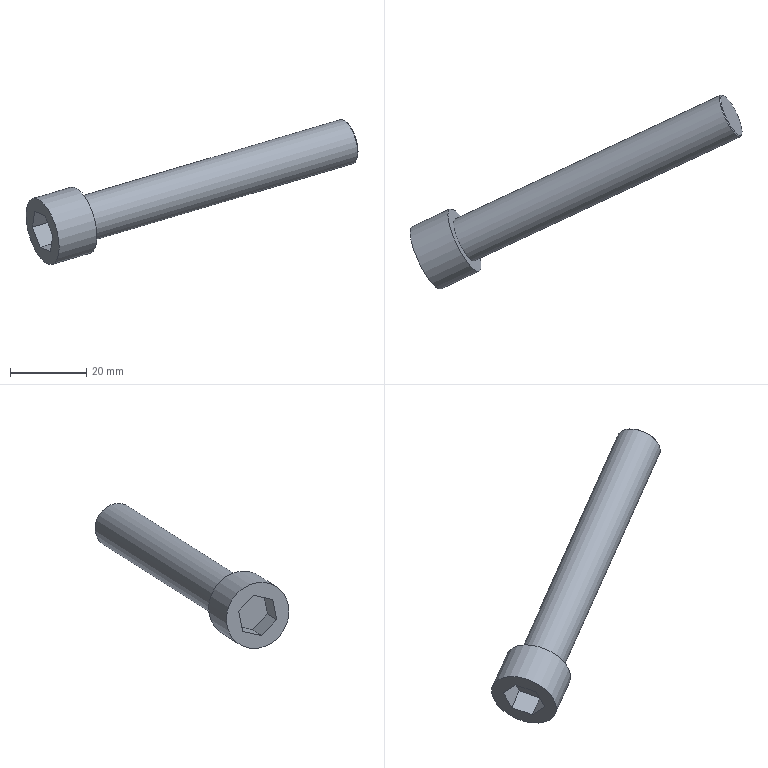Part | NX | features solid 2 | 1 solid | 13 faces | box 87.085 x 50.875 x 38.063 mm | volume 11411 mm3 | plane 10 | cylinder 2 | cone 1 | commonest cylinder face diameters 12 x1 18 x1
STEP:
#1=CARTESIAN_POINT('',(858.778,690.311,-120.934));
#2=VERTEX_POINT('',#1);
#3=CARTESIAN_POINT('',(854.975,698.468,-120.934));
#4=DIRECTION('',(-0.8754,-0.4082,-0.2588));
#5=DIRECTION('',(0.4226,-0.9063,-0.000000003));
#6=AXIS2_PLACEMENT_3D('',#3,#4,#5);
#7=CIRCLE('',#6,9.);
#8=EDGE_CURVE('',#2,#2,#7,.T.);
#9=ORIENTED_EDGE('',*,*,#8,.T.);
#10=EDGE_LOOP('',(#9));
#11=FACE_BOUND('',#10,.T.);
#12=CARTESIAN_POINT('',(854.361,702.423,-125.095));
#13=VERTEX_POINT('',#12);
#14=CARTESIAN_POINT('',(857.025,697.429,-126.23));
#15=VERTEX_POINT('',#14);
#16=CARTESIAN_POINT('',(854.361,702.423,-125.095));
#17=DIRECTION('',(0.4615,-0.8651,-0.1966));
#18=VECTOR('',#17,1000.);
#19=LINE('',#16,#18);
#20=EDGE_CURVE('',#13,#15,#19,.T.);
#21=ORIENTED_EDGE('',*,*,#20,.F.);
#22=CARTESIAN_POINT('',(852.31,703.463,-119.798));
#23=VERTEX_POINT('',#22);
#24=CARTESIAN_POINT('',(852.31,703.463,-119.798));
#25=DIRECTION('',(0.3552,-0.18,-0.9173));
#26=VECTOR('',#25,1000.);
#27=LINE('',#24,#26);
#28=EDGE_CURVE('',#23,#13,#27,.T.);
#29=ORIENTED_EDGE('',*,*,#28,.F.);
#30=CARTESIAN_POINT('',(852.924,699.508,-115.638));
#31=VERTEX_POINT('',#30);
#32=CARTESIAN_POINT('',(852.924,699.508,-115.638));
#33=DIRECTION('',(-0.1064,0.685,-0.7207));
#34=VECTOR('',#33,1000.);
#35=LINE('',#32,#34);
#36=EDGE_CURVE('',#31,#23,#35,.T.);
#37=ORIENTED_EDGE('',*,*,#36,.F.);
#38=CARTESIAN_POINT('',(855.589,694.513,-116.773));
#39=VERTEX_POINT('',#38);
#40=CARTESIAN_POINT('',(855.589,694.513,-116.773));
#41=DIRECTION('',(-0.4615,0.8651,0.1966));
#42=VECTOR('',#41,1000.);
#43=LINE('',#40,#42);
#44=EDGE_CURVE('',#39,#31,#43,.T.);
#45=ORIENTED_EDGE('',*,*,#44,.F.);
#46=CARTESIAN_POINT('',(857.639,693.474,-122.069));
#47=VERTEX_POINT('',#46);
#48=CARTESIAN_POINT('',(857.639,693.474,-122.069));
#49=DIRECTION('',(-0.3552,0.18,0.9173));
#50=VECTOR('',#49,1000.);
#51=LINE('',#48,#50);
#52=EDGE_CURVE('',#47,#39,#51,.T.);
#53=ORIENTED_EDGE('',*,*,#52,.F.);
#54=CARTESIAN_POINT('',(857.025,697.429,-126.23));
#55=DIRECTION('',(0.1064,-0.685,0.7207));
#56=VECTOR('',#55,1000.);
#57=LINE('',#54,#56);
#58=EDGE_CURVE('',#15,#47,#57,.T.);
#59=ORIENTED_EDGE('',*,*,#58,.F.);
#60=EDGE_LOOP('',(#21,#29,#37,#45,#53,#59));
#61=FACE_BOUND('',#60,.T.);
#62=CARTESIAN_POINT('',(854.975,698.468,-120.934));
#63=DIRECTION('',(-0.8754,-0.4082,-0.2588));
#64=DIRECTION('',(-0.4226,0.9063,0.000000003));
#65=AXIS2_PLACEMENT_3D('',#62,#63,#64);
#66=PLANE('',#65);
#67=ADVANCED_FACE('',(#11,#61),#66,.T.);
#68=CARTESIAN_POINT('',(867.432,697.657,-118.));
#69=VERTEX_POINT('',#68);
#70=CARTESIAN_POINT('',(864.896,703.095,-118.));
#71=DIRECTION('',(-0.8754,-0.4082,-0.2588));
#72=DIRECTION('',(0.4226,-0.9063,-0.000000003));
#73=AXIS2_PLACEMENT_3D('',#70,#71,#72);
#74=CIRCLE('',#73,6.);
#75=EDGE_CURVE('',#69,#69,#74,.T.);
#76=ORIENTED_EDGE('',*,*,#75,.T.);
#77=EDGE_LOOP('',(#76));
#78=FACE_BOUND('',#77,.T.);
#79=CARTESIAN_POINT('',(861.093,711.251,-118.));
#80=VERTEX_POINT('',#79);
#81=CARTESIAN_POINT('',(864.896,703.095,-118.));
#82=DIRECTION('',(0.8754,0.4082,0.2588));
#83=DIRECTION('',(-0.4226,0.9063,0.000000003));
#84=AXIS2_PLACEMENT_3D('',#81,#82,#83);
#85=CIRCLE('',#84,9.);
#86=EDGE_CURVE('',#80,#80,#85,.T.);
#87=ORIENTED_EDGE('',*,*,#86,.T.);
#88=EDGE_LOOP('',(#87));
#89=FACE_BOUND('',#88,.T.);
#90=CARTESIAN_POINT('',(864.896,703.095,-118.));
#91=DIRECTION('',(0.8754,0.4082,0.2588));
#92=DIRECTION('',(0.4226,-0.9063,-0.000000003));
#93=AXIS2_PLACEMENT_3D('',#90,#91,#92);
#94=PLANE('',#93);
#95=ADVANCED_FACE('',(#78,#89),#94,.T.);
#96=ORIENTED_EDGE('',*,*,#8,.F.);
#97=EDGE_LOOP('',(#96));
#98=FACE_BOUND('',#97,.T.);
#99=ORIENTED_EDGE('',*,*,#86,.F.);
#100=EDGE_LOOP('',(#99));
#101=FACE_BOUND('',#100,.T.);
#102=CARTESIAN_POINT('',(864.896,703.095,-118.));
#103=DIRECTION('',(-0.8754,-0.4082,-0.2588));
#104=DIRECTION('',(-0.4226,0.9063,0.000000003));
#105=AXIS2_PLACEMENT_3D('',#102,#103,#104);
#106=CYLINDRICAL_SURFACE('',#105,9.);
#107=ADVANCED_FACE('',(#98,#101),#106,.T.);
#108=CARTESIAN_POINT('',(937.361,730.541,-97.295));
#109=VERTEX_POINT('',#108);
#110=CARTESIAN_POINT('',(934.93,735.752,-97.295));
#111=DIRECTION('',(-0.8754,-0.4082,-0.2588));
#112=DIRECTION('',(0.4226,-0.9063,-0.000000003));
#113=AXIS2_PLACEMENT_3D('',#110,#111,#112);
#114=CIRCLE('',#113,5.75);
#115=EDGE_CURVE('',#109,#109,#114,.T.);
#116=ORIENTED_EDGE('',*,*,#115,.F.);
#117=EDGE_LOOP('',(#116));
#118=FACE_BOUND('',#117,.T.);
#119=CARTESIAN_POINT('',(934.93,735.752,-97.295));
#120=DIRECTION('',(0.8754,0.4082,0.2588));
#121=DIRECTION('',(0.4226,-0.9063,-0.000000003));
#122=AXIS2_PLACEMENT_3D('',#119,#120,#121);
#123=PLANE('',#122);
#124=ADVANCED_FACE('',(#118),#123,.T.);
#125=CARTESIAN_POINT('',(937.247,730.212,-97.359));
#126=VERTEX_POINT('',#125);
#127=CARTESIAN_POINT('',(934.712,735.65,-97.359));
#128=DIRECTION('',(-0.8754,-0.4082,-0.2588));
#129=DIRECTION('',(0.4226,-0.9063,-0.000000003));
#130=AXIS2_PLACEMENT_3D('',#127,#128,#129);
#131=CIRCLE('',#130,6.);
#132=EDGE_CURVE('',#126,#126,#131,.F.);
#133=ORIENTED_EDGE('',*,*,#132,.F.);
#134=EDGE_LOOP('',(#133));
#135=FACE_BOUND('',#134,.T.);
#136=ORIENTED_EDGE('',*,*,#75,.F.);
#137=EDGE_LOOP('',(#136));
#138=FACE_BOUND('',#137,.T.);
#139=CARTESIAN_POINT('',(838.634,690.848,-125.765));
#140=DIRECTION('',(0.8754,0.4082,0.2588));
#141=DIRECTION('',(0.4226,-0.9063,-0.000000003));
#142=AXIS2_PLACEMENT_3D('',#139,#140,#141);
#143=CYLINDRICAL_SURFACE('',#142,6.);
#144=ADVANCED_FACE('',(#135,#138),#143,.T.);
#145=ORIENTED_EDGE('',*,*,#132,.T.);
#146=EDGE_LOOP('',(#145));
#147=FACE_BOUND('',#146,.T.);
#148=ORIENTED_EDGE('',*,*,#115,.T.);
#149=EDGE_LOOP('',(#148));
#150=FACE_BOUND('',#149,.T.);
#151=CARTESIAN_POINT('',(934.93,735.752,-97.295));
#152=DIRECTION('',(-0.8754,-0.4082,-0.2588));
#153=DIRECTION('',(-0.4226,0.9063,0.000000003));
#154=AXIS2_PLACEMENT_3D('',#151,#152,#153);
#155=CONICAL_SURFACE('',#154,5.75,0.7854);
#156=ADVANCED_FACE('',(#147,#150),#155,.T.);
#157=ORIENTED_EDGE('',*,*,#58,.T.);
#158=CARTESIAN_POINT('',(862.892,695.923,-120.516));
#159=VERTEX_POINT('',#158);
#160=CARTESIAN_POINT('',(862.892,695.923,-120.516));
#161=DIRECTION('',(-0.8754,-0.4082,-0.2588));
#162=VECTOR('',#161,1000.);
#163=LINE('',#160,#162);
#164=EDGE_CURVE('',#159,#47,#163,.T.);
#165=ORIENTED_EDGE('',*,*,#164,.F.);
#166=CARTESIAN_POINT('',(862.278,699.878,-124.677));
#167=VERTEX_POINT('',#166);
#168=CARTESIAN_POINT('',(862.278,699.878,-124.677));
#169=DIRECTION('',(0.1064,-0.685,0.7207));
#170=VECTOR('',#169,1000.);
#171=LINE('',#168,#170);
#172=EDGE_CURVE('',#167,#159,#171,.T.);
#173=ORIENTED_EDGE('',*,*,#172,.F.);
#174=CARTESIAN_POINT('',(862.278,699.878,-124.677));
#175=DIRECTION('',(-0.8754,-0.4082,-0.2588));
#176=VECTOR('',#175,1000.);
#177=LINE('',#174,#176);
#178=EDGE_CURVE('',#167,#15,#177,.T.);
#179=ORIENTED_EDGE('',*,*,#178,.T.);
#180=EDGE_LOOP('',(#157,#165,#173,#179));
#181=FACE_BOUND('',#180,.T.);
#182=CARTESIAN_POINT('',(862.278,699.878,-124.677));
#183=DIRECTION('',(-0.4715,0.6034,0.6431));
#184=DIRECTION('',(0.1064,-0.685,0.7207));
#185=AXIS2_PLACEMENT_3D('',#182,#183,#184);
#186=PLANE('',#185);
#187=ADVANCED_FACE('',(#181),#186,.T.);
#188=ORIENTED_EDGE('',*,*,#52,.T.);
#189=CARTESIAN_POINT('',(860.842,696.962,-115.22));
#190=VERTEX_POINT('',#189);
#191=CARTESIAN_POINT('',(860.842,696.962,-115.22));
#192=DIRECTION('',(-0.8754,-0.4082,-0.2588));
#193=VECTOR('',#192,1000.);
#194=LINE('',#191,#193);
#195=EDGE_CURVE('',#190,#39,#194,.T.);
#196=ORIENTED_EDGE('',*,*,#195,.F.);
#197=CARTESIAN_POINT('',(862.892,695.923,-120.516));
#198=DIRECTION('',(-0.3552,0.18,0.9173));
#199=VECTOR('',#198,1000.);
#200=LINE('',#197,#199);
#201=EDGE_CURVE('',#159,#190,#200,.T.);
#202=ORIENTED_EDGE('',*,*,#201,.F.);
#203=ORIENTED_EDGE('',*,*,#164,.T.);
#204=EDGE_LOOP('',(#188,#196,#202,#203));
#205=FACE_BOUND('',#204,.T.);
#206=CARTESIAN_POINT('',(862.892,695.923,-120.516));
#207=DIRECTION('',(-0.3279,0.895,-0.3026));
#208=DIRECTION('',(-0.3552,0.18,0.9173));
#209=AXIS2_PLACEMENT_3D('',#206,#207,#208);
#210=PLANE('',#209);
#211=ADVANCED_FACE('',(#205),#210,.T.);
#212=ORIENTED_EDGE('',*,*,#44,.T.);
#213=CARTESIAN_POINT('',(858.177,701.957,-114.085));
#214=VERTEX_POINT('',#213);
#215=CARTESIAN_POINT('',(858.177,701.957,-114.085));
#216=DIRECTION('',(-0.8754,-0.4082,-0.2588));
#217=VECTOR('',#216,1000.);
#218=LINE('',#215,#217);
#219=EDGE_CURVE('',#214,#31,#218,.T.);
#220=ORIENTED_EDGE('',*,*,#219,.F.);
#221=CARTESIAN_POINT('',(860.842,696.962,-115.22));
#222=DIRECTION('',(-0.4615,0.8651,0.1966));
#223=VECTOR('',#222,1000.);
#224=LINE('',#221,#223);
#225=EDGE_CURVE('',#190,#214,#224,.T.);
#226=ORIENTED_EDGE('',*,*,#225,.F.);
#227=ORIENTED_EDGE('',*,*,#195,.T.);
#228=EDGE_LOOP('',(#212,#220,#226,#227));
#229=FACE_BOUND('',#228,.T.);
#230=CARTESIAN_POINT('',(860.842,696.962,-115.22));
#231=DIRECTION('',(0.1436,0.2916,-0.9457));
#232=DIRECTION('',(-0.4615,0.8651,0.1966));
#233=AXIS2_PLACEMENT_3D('',#230,#231,#232);
#234=PLANE('',#233);
#235=ADVANCED_FACE('',(#229),#234,.T.);
#236=ORIENTED_EDGE('',*,*,#36,.T.);
#237=CARTESIAN_POINT('',(857.563,705.912,-118.246));
#238=VERTEX_POINT('',#237);
#239=CARTESIAN_POINT('',(857.563,705.912,-118.246));
#240=DIRECTION('',(-0.8754,-0.4082,-0.2588));
#241=VECTOR('',#240,1000.);
#242=LINE('',#239,#241);
#243=EDGE_CURVE('',#238,#23,#242,.T.);
#244=ORIENTED_EDGE('',*,*,#243,.F.);
#245=CARTESIAN_POINT('',(858.177,701.957,-114.085));
#246=DIRECTION('',(-0.1064,0.685,-0.7207));
#247=VECTOR('',#246,1000.);
#248=LINE('',#245,#247);
#249=EDGE_CURVE('',#214,#238,#248,.T.);
#250=ORIENTED_EDGE('',*,*,#249,.F.);
#251=ORIENTED_EDGE('',*,*,#219,.T.);
#252=EDGE_LOOP('',(#236,#244,#250,#251));
#253=FACE_BOUND('',#252,.T.);
#254=CARTESIAN_POINT('',(858.177,701.957,-114.085));
#255=DIRECTION('',(0.4715,-0.6034,-0.6431));
#256=DIRECTION('',(-0.1064,0.685,-0.7207));
#257=AXIS2_PLACEMENT_3D('',#254,#255,#256);
#258=PLANE('',#257);
#259=ADVANCED_FACE('',(#253),#258,.T.);
#260=ORIENTED_EDGE('',*,*,#28,.T.);
#261=CARTESIAN_POINT('',(859.613,704.873,-123.542));
#262=VERTEX_POINT('',#261);
#263=CARTESIAN_POINT('',(859.613,704.873,-123.542));
#264=DIRECTION('',(-0.8754,-0.4082,-0.2588));
#265=VECTOR('',#264,1000.);
#266=LINE('',#263,#265);
#267=EDGE_CURVE('',#262,#13,#266,.T.);
#268=ORIENTED_EDGE('',*,*,#267,.F.);
#269=CARTESIAN_POINT('',(857.563,705.912,-118.246));
#270=DIRECTION('',(0.3552,-0.18,-0.9173));
#271=VECTOR('',#270,1000.);
#272=LINE('',#269,#271);
#273=EDGE_CURVE('',#238,#262,#272,.T.);
#274=ORIENTED_EDGE('',*,*,#273,.F.);
#275=ORIENTED_EDGE('',*,*,#243,.T.);
#276=EDGE_LOOP('',(#260,#268,#274,#275));
#277=FACE_BOUND('',#276,.T.);
#278=CARTESIAN_POINT('',(857.563,705.912,-118.246));
#279=DIRECTION('',(0.3279,-0.895,0.3026));
#280=DIRECTION('',(0.3552,-0.18,-0.9173));
#281=AXIS2_PLACEMENT_3D('',#278,#279,#280);
#282=PLANE('',#281);
#283=ADVANCED_FACE('',(#277),#282,.T.);
#284=ORIENTED_EDGE('',*,*,#20,.T.);
#285=ORIENTED_EDGE('',*,*,#178,.F.);
#286=CARTESIAN_POINT('',(859.613,704.873,-123.542));
#287=DIRECTION('',(0.4615,-0.8651,-0.1966));
#288=VECTOR('',#287,1000.);
#289=LINE('',#286,#288);
#290=EDGE_CURVE('',#262,#167,#289,.T.);
#291=ORIENTED_EDGE('',*,*,#290,.F.);
#292=ORIENTED_EDGE('',*,*,#267,.T.);
#293=EDGE_LOOP('',(#284,#285,#291,#292));
#294=FACE_BOUND('',#293,.T.);
#295=CARTESIAN_POINT('',(859.613,704.873,-123.542));
#296=DIRECTION('',(-0.1436,-0.2916,0.9457));
#297=DIRECTION('',(0.4615,-0.8651,-0.1966));
#298=AXIS2_PLACEMENT_3D('',#295,#296,#297);
#299=PLANE('',#298);
#300=ADVANCED_FACE('',(#294),#299,.T.);
#301=ORIENTED_EDGE('',*,*,#172,.T.);
#302=ORIENTED_EDGE('',*,*,#201,.T.);
#303=ORIENTED_EDGE('',*,*,#225,.T.);
#304=ORIENTED_EDGE('',*,*,#249,.T.);
#305=ORIENTED_EDGE('',*,*,#273,.T.);
#306=ORIENTED_EDGE('',*,*,#290,.T.);
#307=EDGE_LOOP('',(#301,#302,#303,#304,#305,#306));
#308=FACE_BOUND('',#307,.T.);
#309=CARTESIAN_POINT('',(862.892,695.923,-120.516));
#310=DIRECTION('',(0.8754,0.4082,0.2588));
#311=DIRECTION('',(0.4226,-0.9063,-0.000000003));
#312=AXIS2_PLACEMENT_3D('',#309,#310,#311);
#313=PLANE('',#312);
#314=ADVANCED_FACE('',(#308),#313,.F.);
#315=CLOSED_SHELL('',(#67,#95,#107,#124,#144,#156,#187,#211,#235,#259,#283,#300,#314));
#316=MANIFOLD_SOLID_BREP('',#315);
#317=(LENGTH_UNIT()NAMED_UNIT(*)SI_UNIT(.MILLI.,.METRE.));
#318=UNCERTAINTY_MEASURE_WITH_UNIT(LENGTH_MEASURE(0.00001),#317,'','');
#319=(NAMED_UNIT(*)PLANE_ANGLE_UNIT()SI_UNIT($,.RADIAN.));
#320=(NAMED_UNIT(*)SI_UNIT($,.STERADIAN.)SOLID_ANGLE_UNIT());
#321=(GEOMETRIC_REPRESENTATION_CONTEXT(3)GLOBAL_UNCERTAINTY_ASSIGNED_CONTEXT((#318))GLOBAL_UNIT_ASSIGNED_CONTEXT((#317,#319,#320))REPRESENTATION_CONTEXT('',''));
#322=ADVANCED_BREP_SHAPE_REPRESENTATION('',(#316),#321);